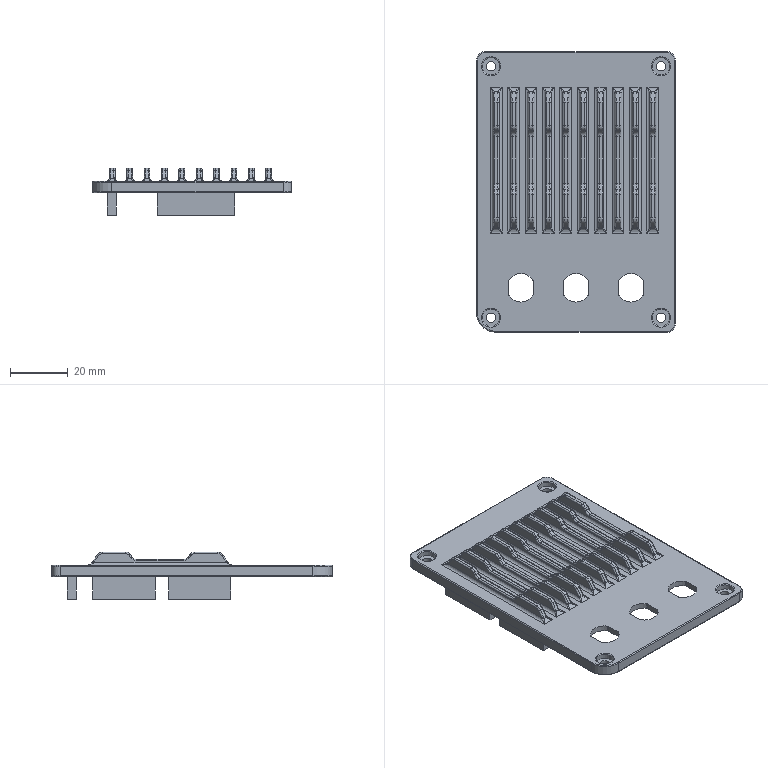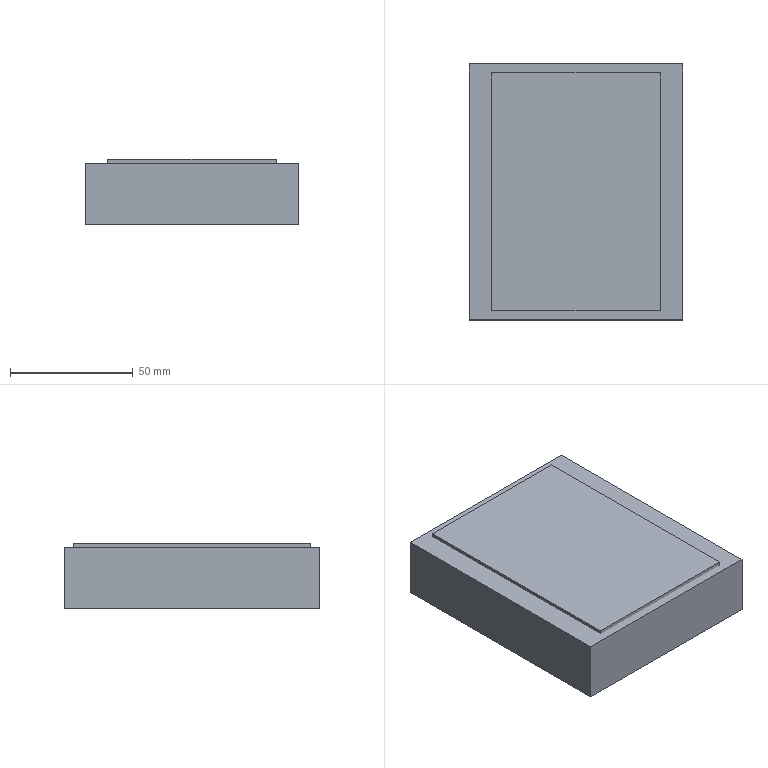CAM job | NX | 3-axis milling | part box 68.665 x 96.782 x 16.5 mm | stock box 86.883 x 104.117 x 26.5 mm
Tools:
number,name,description,diameter,corner_radius,flute_length,length,flutes
5,D2平刀,Milling Tool-5 Parameters,1.5,0.0,50.0,75.0,2
1,D8平刀,Milling Tool-5 Parameters,8.0,0.0,50.0,75.0,2
2,D3平刀,Milling Tool-5 Parameters,3.0,0.0,50.0,75.0,2
3,倒角刀,Milling Tool-5 Parameters,3.0,0.0,50.0,75.0,2
4,R1,Milling Tool-5 Parameters,2.0,1.0,50.0,75.0,2
Operations:
program,operation,operation_type,tool,method,geometry_group,spindle_rpm,surface_speed,feed_per_tooth,feed_cut,feed_plunge,cut_length_mm,path_length_mm,cut_time_min,machine_time_min
G54,ADAPTIVE_MILLING,CavityMilling,D8平刀,METHOD,WORKPIECE,5500.0,138.0,0.2273,2500.0,100.0,11764.658,12156.61,4.567,4.606
G54,PLANAR_MILL_5,PlanarMilling,D8平刀,METHOD,WORKPIECE,4000.0,100.0,0.1,800.0,100.0,133.963,246.041,0.1675,0.1787
G54,PLANAR_MILL_2,PlanarMilling,D8平刀,METHOD,WORKPIECE,4000.0,100.0,0.1,800.0,100.0,361.787,431.787,0.4522,0.4592
G54,PLANAR_MILL_4,PlanarMilling,D8平刀,METHOD,WORKPIECE,4000.0,100.0,0.1,800.0,100.0,689.787,739.787,0.8622,0.8672
G54,PLANAR_MILL_3,PlanarMilling,D8平刀,METHOD,WORKPIECE,4000.0,100.0,0.1,800.0,100.0,1432.307,1491.307,1.79,1.796
G54,PLANAR_MILL,PlanarMilling,D3平刀,METHOD,WORKPIECE,4500.0,42.0,0.2222,2000.0,100.0,3661.128,3869.172,1.831,1.851
G54,PLANAR_MILL_COPY,PlanarMilling,D3平刀,METHOD,WORKPIECE,4500.0,42.0,0.0667,600.0,100.0,865.538,1706.383,1.443,1.527
G54,PLANAR_MILL_1,PlanarMilling,D3平刀,METHOD,WORKPIECE,4500.0,42.0,0.1111,1000.0,100.0,991.036,1221.032,0.991,1.014
G54,PLANAR_MILL_1_COPY,PlanarMilling,D3平刀,METHOD,WORKPIECE,3500.0,32.0,0.0857,600.0,100.0,86.859,306.485,0.1448,0.1667
G54,PLANAR_MILL_3_COPY,PlanarMilling,D3平刀,METHOD,WORKPIECE,3500.0,32.0,0.0857,600.0,100.0,1393.236,2144.954,2.322,2.397
G54,PLANAR_MILL_3_COPY_COPY,PlanarMilling,D3平刀,METHOD,WORKPIECE,3500.0,32.0,0.0857,600.0,100.0,347.454,1047.863,0.5791,0.6491
G54,PLANAR_MILL_COPY_1,PlanarMilling,倒角刀,METHOD,WORKPIECE,4500.0,42.0,0.2222,1000.0,100.0,204.474,393.759,0.2045,0.2234
G54,PLANAR_MILL_2_COPY,PlanarMilling,倒角刀,METHOD,WORKPIECE,4500.0,42.0,0.2222,1000.0,100.0,342.309,394.309,0.3423,0.3475
G54,PLANAR_MILL_6,PlanarMilling,倒角刀,METHOD,WORKPIECE,4500.0,42.0,0.2222,1000.0,100.0,306.956,358.956,0.307,0.3122
G54,PLANAR_MILL_7,PlanarMilling,倒角刀,METHOD,WORKPIECE,4500.0,42.0,0.2222,1000.0,100.0,102.052,312.857,0.1021,0.1231
G55,CAVITY_MILL,CavityMilling,D8平刀,METHOD,WORKPIECE_1,5500.0,138.0,0.2727,3000.0,100.0,13574.07,16378.07,4.525,4.805
G55,FLOOR_WALL,VolumeBased25DMillingOperation,D8平刀,METHOD,WORKPIECE_1,3500.0,87.0,0.1143,800.0,100.0,601.319,779.506,0.7516,0.7695
G55,CAVITY_MILL_COPY,CavityMilling,D3平刀,METHOD,WORKPIECE_1,5500.0,51.0,0.1818,2000.0,100.0,14818.603,19373.811,7.409,7.865
G55,PLANAR_MILL_8_COPY,PlanarMilling,D3平刀,METHOD,WORKPIECE_1,4500.0,100.0,0.1178,200.0,100.0,284.987,676.057,1.425,1.464
G55,PLANAR_MILL_1_COPY_1,PlanarMilling,D3平刀,METHOD,WORKPIECE_1,4500.0,42.0,0.1111,1000.0,100.0,1423.561,1820.819,1.424,1.463
G55,FLOOR_WALL_COPY,VolumeBased25DMillingOperation,D2平刀,METHOD,WORKPIECE_1,3500.0,16.0,0.1143,800.0,100.0,1682.492,2320.49,2.103,2.167
G55,PLANAR_MILL_1_COPY_1_COPY,PlanarMilling,D2平刀,METHOD,WORKPIECE_1,4500.0,42.0,0.1111,1000.0,100.0,2553.153,2956.082,2.553,2.593
G55,PLANAR_MILL_8,PlanarMilling,D2平刀,METHOD,WORKPIECE_1,4500.0,21.0,0.0222,200.0,100.0,51.363,463.476,0.2568,0.298
G55,AREA_MILL_COPY,SurfaceContour,R1,METHOD,WORKPIECE_1,5500.0,34.0,0.2727,3000.0,100.0,62726.411,71720.606,20.909,21.808
G55,AREA_MILL_COPY_COPY,SurfaceContour,R1,METHOD,WORKPIECE_1,5500.0,34.0,0.2727,3000.0,100.0,11975.656,13463.459,3.992,4.141
G55,PLANAR_MILL_8_COPY_1,PlanarMilling,倒角刀,METHOD,WORKPIECE_1,4500.0,21.0,0.0222,200.0,100.0,105.397,280.697,0.527,0.5445